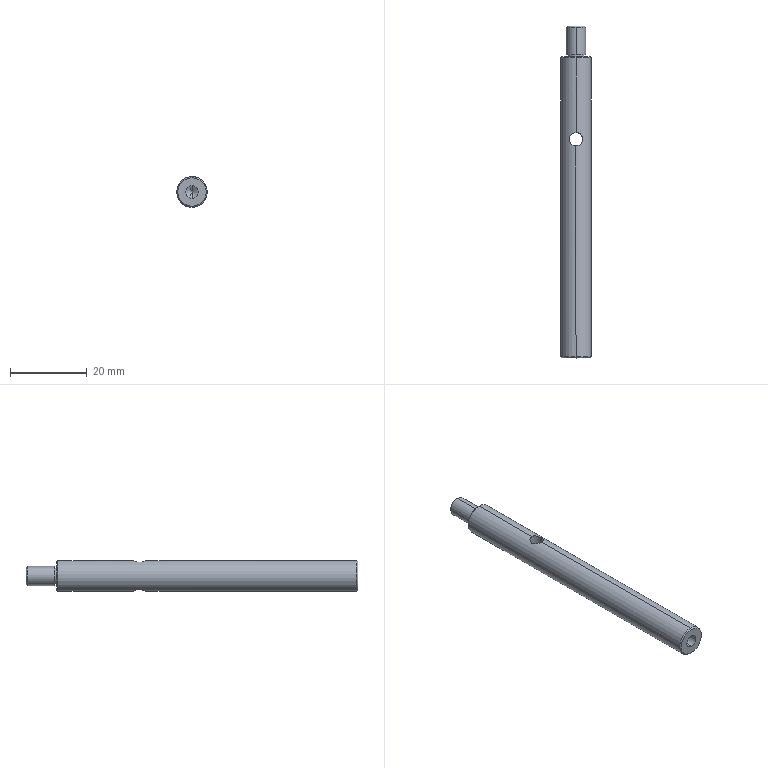Part | SolidWorks | features ICE 2, Chamfer 1, Extrusion 1, HoleWzd 1, RevCut 1 | 1 solid | 22 faces | box 8 x 86.5 x 8 mm | volume 3934 mm3 | cylinder 10 | cone 8 | plane 4 | commonest cylinder face diameters 3.3 x2 3.5 x2 4.4 x2 5 x2 8 x2
STEP:
#1=CARTESIAN_POINT('',(0.,86.2,-2.5));
#2=VERTEX_POINT('',#1);
#3=CARTESIAN_POINT('',(0.,86.2,2.5));
#4=VERTEX_POINT('',#3);
#5=CARTESIAN_POINT('',(0.,86.2,0.));
#6=DIRECTION('',(0.,-1.,0.));
#7=DIRECTION('',(0.,0.,1.));
#8=AXIS2_PLACEMENT_3D('',#5,#6,#7);
#9=CIRCLE('',#8,2.5);
#10=EDGE_CURVE('',#2,#4,#9,.T.);
#11=ORIENTED_EDGE('',*,*,#10,.T.);
#12=CARTESIAN_POINT('',(0.,79.,2.5));
#13=VERTEX_POINT('',#12);
#14=CARTESIAN_POINT('',(0.,86.5,2.5));
#15=DIRECTION('',(0.,-1.,0.));
#16=VECTOR('',#15,1000.);
#17=LINE('',#14,#16);
#18=EDGE_CURVE('',#4,#13,#17,.T.);
#19=ORIENTED_EDGE('',*,*,#18,.T.);
#20=CARTESIAN_POINT('',(0.,79.,-2.5));
#21=VERTEX_POINT('',#20);
#22=CARTESIAN_POINT('',(0.,79.,0.));
#23=DIRECTION('',(0.,-1.,0.));
#24=DIRECTION('',(0.,0.,-1.));
#25=AXIS2_PLACEMENT_3D('',#22,#23,#24);
#26=CIRCLE('',#25,2.5);
#27=EDGE_CURVE('',#21,#13,#26,.T.);
#28=ORIENTED_EDGE('',*,*,#27,.F.);
#29=CARTESIAN_POINT('',(0.,86.5,-2.5));
#30=DIRECTION('',(0.,-1.,0.));
#31=VECTOR('',#30,1000.);
#32=LINE('',#29,#31);
#33=EDGE_CURVE('',#2,#21,#32,.T.);
#34=ORIENTED_EDGE('',*,*,#33,.F.);
#35=EDGE_LOOP('',(#11,#19,#28,#34));
#36=FACE_OUTER_BOUND('',#35,.T.);
#37=CARTESIAN_POINT('',(0.,86.5,0.));
#38=DIRECTION('',(0.,-1.,0.));
#39=DIRECTION('',(0.,0.,-1.));
#40=AXIS2_PLACEMENT_3D('',#37,#38,#39);
#41=CYLINDRICAL_SURFACE('',#40,2.5);
#42=ADVANCED_FACE('',(#36),#41,.T.);
#43=CARTESIAN_POINT('',(0.,86.5,2.2));
#44=VERTEX_POINT('',#43);
#45=CARTESIAN_POINT('',(0.,86.5,-2.2));
#46=VERTEX_POINT('',#45);
#47=CARTESIAN_POINT('',(0.,86.5,0.));
#48=DIRECTION('',(0.,1.,0.));
#49=DIRECTION('',(0.,0.,1.));
#50=AXIS2_PLACEMENT_3D('',#47,#48,#49);
#51=CIRCLE('',#50,2.2);
#52=EDGE_CURVE('',#44,#46,#51,.T.);
#53=ORIENTED_EDGE('',*,*,#52,.F.);
#54=CARTESIAN_POINT('',(0.,86.5,2.2));
#55=DIRECTION('',(0.,-0.7071,0.7071));
#56=VECTOR('',#55,1000.);
#57=LINE('',#54,#56);
#58=EDGE_CURVE('',#44,#4,#57,.T.);
#59=ORIENTED_EDGE('',*,*,#58,.T.);
#60=ORIENTED_EDGE('',*,*,#10,.F.);
#61=CARTESIAN_POINT('',(0.,86.5,-2.2));
#62=DIRECTION('',(0.,-0.7071,-0.7071));
#63=VECTOR('',#62,1000.);
#64=LINE('',#61,#63);
#65=EDGE_CURVE('',#46,#2,#64,.T.);
#66=ORIENTED_EDGE('',*,*,#65,.F.);
#67=EDGE_LOOP('',(#53,#59,#60,#66));
#68=FACE_OUTER_BOUND('',#67,.T.);
#69=CARTESIAN_POINT('',(0.,86.5,0.));
#70=DIRECTION('',(0.,-1.,0.));
#71=DIRECTION('',(0.,0.,-1.));
#72=AXIS2_PLACEMENT_3D('',#69,#70,#71);
#73=CONICAL_SURFACE('',#72,2.2,0.7854);
#74=ADVANCED_FACE('',(#68),#73,.T.);
#75=CARTESIAN_POINT('',(0.,79.,-2.2));
#76=VERTEX_POINT('',#75);
#77=CARTESIAN_POINT('',(0.,79.,2.2));
#78=VERTEX_POINT('',#77);
#79=CARTESIAN_POINT('',(0.,79.,0.));
#80=DIRECTION('',(0.,-1.,0.));
#81=DIRECTION('',(0.,0.,-1.));
#82=AXIS2_PLACEMENT_3D('',#79,#80,#81);
#83=CIRCLE('',#82,2.2);
#84=EDGE_CURVE('',#76,#78,#83,.T.);
#85=ORIENTED_EDGE('',*,*,#84,.T.);
#86=CARTESIAN_POINT('',(0.,78.5,2.2));
#87=VERTEX_POINT('',#86);
#88=CARTESIAN_POINT('',(0.,0.,2.2));
#89=DIRECTION('',(0.,-1.,0.));
#90=VECTOR('',#89,1000.);
#91=LINE('',#88,#90);
#92=EDGE_CURVE('',#78,#87,#91,.T.);
#93=ORIENTED_EDGE('',*,*,#92,.T.);
#94=CARTESIAN_POINT('',(0.,78.5,-2.2));
#95=VERTEX_POINT('',#94);
#96=CARTESIAN_POINT('',(0.,78.5,0.));
#97=DIRECTION('',(0.,-1.,0.));
#98=DIRECTION('',(0.,0.,-1.));
#99=AXIS2_PLACEMENT_3D('',#96,#97,#98);
#100=CIRCLE('',#99,2.2);
#101=EDGE_CURVE('',#95,#87,#100,.T.);
#102=ORIENTED_EDGE('',*,*,#101,.F.);
#103=CARTESIAN_POINT('',(0.,0.,-2.2));
#104=DIRECTION('',(0.,-1.,0.));
#105=VECTOR('',#104,1000.);
#106=LINE('',#103,#105);
#107=EDGE_CURVE('',#76,#95,#106,.T.);
#108=ORIENTED_EDGE('',*,*,#107,.F.);
#109=EDGE_LOOP('',(#85,#93,#102,#108));
#110=FACE_OUTER_BOUND('',#109,.T.);
#111=CARTESIAN_POINT('',(0.,0.,0.));
#112=DIRECTION('',(0.,-1.,0.));
#113=DIRECTION('',(0.,0.,-1.));
#114=AXIS2_PLACEMENT_3D('',#111,#112,#113);
#115=CYLINDRICAL_SURFACE('',#114,2.2);
#116=ADVANCED_FACE('',(#110),#115,.T.);
#117=CARTESIAN_POINT('',(-1.75,57.,-3.597));
#118=VERTEX_POINT('',#117);
#119=CARTESIAN_POINT('',(0.,55.25,-4.));
#120=VERTEX_POINT('',#119);
#121=CARTESIAN_POINT('',(-1.75,57.,-3.597));
#122=CARTESIAN_POINT('',(-1.75,56.884,-3.597));
#123=CARTESIAN_POINT('',(-1.738,56.767,-3.603));
#124=CARTESIAN_POINT('',(-1.693,56.541,-3.624));
#125=CARTESIAN_POINT('',(-1.659,56.431,-3.64));
#126=CARTESIAN_POINT('',(-1.57,56.218,-3.679));
#127=CARTESIAN_POINT('',(-1.516,56.118,-3.702));
#128=CARTESIAN_POINT('',(-1.39,55.93,-3.751));
#129=CARTESIAN_POINT('',(-1.317,55.842,-3.778));
#130=CARTESIAN_POINT('',(-1.157,55.682,-3.83));
#131=CARTESIAN_POINT('',(-1.07,55.61,-3.856));
#132=CARTESIAN_POINT('',(-0.8807,55.483,-3.903));
#133=CARTESIAN_POINT('',(-0.7792,55.429,-3.925));
#134=CARTESIAN_POINT('',(-0.4639,55.297,-3.979));
#135=CARTESIAN_POINT('',(-0.2309,55.25,-4.));
#136=CARTESIAN_POINT('',(0.,55.25,-4.));
#137=B_SPLINE_CURVE_WITH_KNOTS('',3,(#121,#122,#123,#124,#125,#126,#127,#128,#129,#130,#131,#132,#133,#134,#135,#136),.UNSPECIFIED.,.F.,.F.,(4,2,2,2,2,2,2,4),(0.002772,0.003119,0.003465,0.003811,0.004157,0.004504,0.00485,0.005542),.UNSPECIFIED.);
#138=EDGE_CURVE('',#118,#120,#137,.T.);
#139=ORIENTED_EDGE('',*,*,#138,.F.);
#140=CARTESIAN_POINT('',(-1.75,57.,3.597));
#141=VERTEX_POINT('',#140);
#142=CARTESIAN_POINT('',(-1.75,57.,-5.));
#143=DIRECTION('',(0.,0.,1.));
#144=VECTOR('',#143,1000.);
#145=LINE('',#142,#144);
#146=EDGE_CURVE('',#118,#141,#145,.T.);
#147=ORIENTED_EDGE('',*,*,#146,.T.);
#148=CARTESIAN_POINT('',(0.,55.25,4.));
#149=VERTEX_POINT('',#148);
#150=CARTESIAN_POINT('',(0.,55.25,4.));
#151=CARTESIAN_POINT('',(-0.1159,55.25,4.));
#152=CARTESIAN_POINT('',(-0.2333,55.262,3.995));
#153=CARTESIAN_POINT('',(-0.4592,55.307,3.975));
#154=CARTESIAN_POINT('',(-0.5696,55.341,3.961));
#155=CARTESIAN_POINT('',(-0.7826,55.43,3.924));
#156=CARTESIAN_POINT('',(-0.8826,55.485,3.903));
#157=CARTESIAN_POINT('',(-1.071,55.611,3.855));
#158=CARTESIAN_POINT('',(-1.16,55.684,3.829));
#159=CARTESIAN_POINT('',(-1.319,55.844,3.777));
#160=CARTESIAN_POINT('',(-1.39,55.931,3.751));
#161=CARTESIAN_POINT('',(-1.517,56.12,3.702));
#162=CARTESIAN_POINT('',(-1.571,56.222,3.679));
#163=CARTESIAN_POINT('',(-1.703,56.536,3.621));
#164=CARTESIAN_POINT('',(-1.75,56.769,3.597));
#165=CARTESIAN_POINT('',(-1.75,57.,3.597));
#166=B_SPLINE_CURVE_WITH_KNOTS('',3,(#150,#151,#152,#153,#154,#155,#156,#157,#158,#159,#160,#161,#162,#163,#164,#165),.UNSPECIFIED.,.F.,.F.,(4,2,2,2,2,2,2,4),(0.002772,0.003118,0.003464,0.003811,0.004157,0.004503,0.004849,0.005542),.UNSPECIFIED.);
#167=EDGE_CURVE('',#149,#141,#166,.T.);
#168=ORIENTED_EDGE('',*,*,#167,.F.);
#169=CARTESIAN_POINT('',(1.75,57.,3.597));
#170=VERTEX_POINT('',#169);
#171=CARTESIAN_POINT('',(1.75,57.,3.597));
#172=CARTESIAN_POINT('',(1.75,56.883,3.597));
#173=CARTESIAN_POINT('',(1.738,56.768,3.603));
#174=CARTESIAN_POINT('',(1.693,56.542,3.624));
#175=CARTESIAN_POINT('',(1.659,56.43,3.64));
#176=CARTESIAN_POINT('',(1.526,56.113,3.699));
#177=CARTESIAN_POINT('',(1.397,55.922,3.752));
#178=CARTESIAN_POINT('',(1.078,55.603,3.856));
#179=CARTESIAN_POINT('',(0.885,55.473,3.907));
#180=CARTESIAN_POINT('',(0.5694,55.341,3.961));
#181=CARTESIAN_POINT('',(0.4575,55.307,3.975));
#182=CARTESIAN_POINT('',(0.2307,55.261,3.995));
#183=CARTESIAN_POINT('',(0.116,55.25,4.));
#184=CARTESIAN_POINT('',(0.,55.25,4.));
#185=B_SPLINE_CURVE_WITH_KNOTS('',3,(#171,#172,#173,#174,#175,#176,#177,#178,#179,#180,#181,#182,#183,#184),.UNSPECIFIED.,.F.,.F.,(4,2,2,2,2,2,4),(0.,0.0003465,0.000693,0.001386,0.002079,0.002425,0.002772),.UNSPECIFIED.);
#186=EDGE_CURVE('',#170,#149,#185,.T.);
#187=ORIENTED_EDGE('',*,*,#186,.F.);
#188=CARTESIAN_POINT('',(1.75,57.,-3.597));
#189=VERTEX_POINT('',#188);
#190=CARTESIAN_POINT('',(1.75,57.,-5.));
#191=DIRECTION('',(0.,0.,1.));
#192=VECTOR('',#191,1000.);
#193=LINE('',#190,#192);
#194=EDGE_CURVE('',#189,#170,#193,.T.);
#195=ORIENTED_EDGE('',*,*,#194,.F.);
#196=CARTESIAN_POINT('',(0.,55.25,-4.));
#197=CARTESIAN_POINT('',(0.1154,55.25,-4.));
#198=CARTESIAN_POINT('',(0.2327,55.262,-3.995));
#199=CARTESIAN_POINT('',(0.4595,55.307,-3.975));
#200=CARTESIAN_POINT('',(0.5691,55.341,-3.961));
#201=CARTESIAN_POINT('',(0.8874,55.474,-3.906));
#202=CARTESIAN_POINT('',(1.079,55.603,-3.856));
#203=CARTESIAN_POINT('',(1.319,55.844,-3.777));
#204=CARTESIAN_POINT('',(1.391,55.931,-3.751));
#205=CARTESIAN_POINT('',(1.516,56.119,-3.702));
#206=CARTESIAN_POINT('',(1.571,56.221,-3.679));
#207=CARTESIAN_POINT('',(1.659,56.432,-3.64));
#208=CARTESIAN_POINT('',(1.693,56.541,-3.624));
#209=CARTESIAN_POINT('',(1.738,56.767,-3.603));
#210=CARTESIAN_POINT('',(1.75,56.885,-3.597));
#211=CARTESIAN_POINT('',(1.75,57.,-3.597));
#212=B_SPLINE_CURVE_WITH_KNOTS('',3,(#196,#197,#198,#199,#200,#201,#202,#203,#204,#205,#206,#207,#208,#209,#210,#211),.UNSPECIFIED.,.F.,.F.,(4,2,2,2,2,2,2,4),(0.005542,0.005888,0.006235,0.006927,0.007273,0.007619,0.007965,0.008311),.UNSPECIFIED.);
#213=EDGE_CURVE('',#120,#189,#212,.T.);
#214=ORIENTED_EDGE('',*,*,#213,.F.);
#215=EDGE_LOOP('',(#139,#147,#168,#187,#195,#214));
#216=FACE_OUTER_BOUND('',#215,.T.);
#217=CARTESIAN_POINT('',(0.,57.,-5.));
#218=DIRECTION('',(0.,0.,1.));
#219=DIRECTION('',(1.,0.,0.));
#220=AXIS2_PLACEMENT_3D('',#217,#218,#219);
#221=CYLINDRICAL_SURFACE('',#220,1.75);
#222=ADVANCED_FACE('',(#216),#221,.F.);
#223=CARTESIAN_POINT('',(0.,10.1,1.65));
#224=VERTEX_POINT('',#223);
#225=CARTESIAN_POINT('',(0.,10.1,-1.65));
#226=VERTEX_POINT('',#225);
#227=CARTESIAN_POINT('',(0.,10.1,0.));
#228=DIRECTION('',(0.,-1.,0.));
#229=DIRECTION('',(0.,0.,-1.));
#230=AXIS2_PLACEMENT_3D('',#227,#228,#229);
#231=CIRCLE('',#230,1.65);
#232=EDGE_CURVE('',#224,#226,#231,.T.);
#233=ORIENTED_EDGE('',*,*,#232,.F.);
#234=CARTESIAN_POINT('',(0.,0.,1.65));
#235=VERTEX_POINT('',#234);
#236=CARTESIAN_POINT('',(0.,0.,1.65));
#237=DIRECTION('',(0.,-1.,0.));
#238=VECTOR('',#237,1000.);
#239=LINE('',#236,#238);
#240=EDGE_CURVE('',#224,#235,#239,.T.);
#241=ORIENTED_EDGE('',*,*,#240,.T.);
#242=CARTESIAN_POINT('',(0.,0.,-1.65));
#243=VERTEX_POINT('',#242);
#244=CARTESIAN_POINT('',(0.,0.,0.));
#245=DIRECTION('',(0.,-1.,0.));
#246=DIRECTION('',(0.,0.,-1.));
#247=AXIS2_PLACEMENT_3D('',#244,#245,#246);
#248=CIRCLE('',#247,1.65);
#249=EDGE_CURVE('',#235,#243,#248,.T.);
#250=ORIENTED_EDGE('',*,*,#249,.T.);
#251=CARTESIAN_POINT('',(0.,0.,-1.65));
#252=DIRECTION('',(0.,-1.,0.));
#253=VECTOR('',#252,1000.);
#254=LINE('',#251,#253);
#255=EDGE_CURVE('',#226,#243,#254,.T.);
#256=ORIENTED_EDGE('',*,*,#255,.F.);
#257=EDGE_LOOP('',(#233,#241,#250,#256));
#258=FACE_OUTER_BOUND('',#257,.T.);
#259=CARTESIAN_POINT('',(0.,0.,0.));
#260=DIRECTION('',(0.,-1.,0.));
#261=DIRECTION('',(0.,0.,-1.));
#262=AXIS2_PLACEMENT_3D('',#259,#260,#261);
#263=CYLINDRICAL_SURFACE('',#262,1.65);
#264=ADVANCED_FACE('',(#258),#263,.F.);
#265=CARTESIAN_POINT('',(0.,11.091,0.));
#266=VERTEX_POINT('',#265);
#267=CARTESIAN_POINT('',(0.,10.1,-1.65));
#268=DIRECTION('',(0.,-0.515,-0.8572));
#269=VECTOR('',#268,1000.);
#270=LINE('',#267,#269);
#271=EDGE_CURVE('',#266,#226,#270,.T.);
#272=ORIENTED_EDGE('',*,*,#271,.F.);
#273=CARTESIAN_POINT('',(0.,10.1,1.65));
#274=DIRECTION('',(0.,-0.515,0.8572));
#275=VECTOR('',#274,1000.);
#276=LINE('',#273,#275);
#277=EDGE_CURVE('',#266,#224,#276,.T.);
#278=ORIENTED_EDGE('',*,*,#277,.T.);
#279=ORIENTED_EDGE('',*,*,#232,.T.);
#280=EDGE_LOOP('',(#272,#278,#279));
#281=FACE_OUTER_BOUND('',#280,.T.);
#282=CARTESIAN_POINT('',(0.,10.1,0.));
#283=DIRECTION('',(0.,-1.,0.));
#284=DIRECTION('',(0.,0.,-1.));
#285=AXIS2_PLACEMENT_3D('',#282,#283,#284);
#286=CONICAL_SURFACE('',#285,1.65,1.03);
#287=ADVANCED_FACE('',(#281),#286,.F.);
#288=CARTESIAN_POINT('',(0.,78.5,3.7));
#289=VERTEX_POINT('',#288);
#290=CARTESIAN_POINT('',(0.,78.5,-3.7));
#291=VERTEX_POINT('',#290);
#292=CARTESIAN_POINT('',(0.,78.5,0.));
#293=DIRECTION('',(0.,1.,0.));
#294=DIRECTION('',(0.,0.,1.));
#295=AXIS2_PLACEMENT_3D('',#292,#293,#294);
#296=CIRCLE('',#295,3.7);
#297=EDGE_CURVE('',#289,#291,#296,.T.);
#298=ORIENTED_EDGE('',*,*,#297,.F.);
#299=CARTESIAN_POINT('',(0.,78.2,4.));
#300=VERTEX_POINT('',#299);
#301=CARTESIAN_POINT('',(0.,78.5,3.7));
#302=DIRECTION('',(0.,-0.7071,0.7071));
#303=VECTOR('',#302,1000.);
#304=LINE('',#301,#303);
#305=EDGE_CURVE('',#289,#300,#304,.T.);
#306=ORIENTED_EDGE('',*,*,#305,.T.);
#307=CARTESIAN_POINT('',(0.,78.2,-4.));
#308=VERTEX_POINT('',#307);
#309=CARTESIAN_POINT('',(0.,78.2,0.));
#310=DIRECTION('',(0.,-1.,0.));
#311=DIRECTION('',(0.,0.,1.));
#312=AXIS2_PLACEMENT_3D('',#309,#310,#311);
#313=CIRCLE('',#312,4.);
#314=EDGE_CURVE('',#308,#300,#313,.T.);
#315=ORIENTED_EDGE('',*,*,#314,.F.);
#316=CARTESIAN_POINT('',(0.,78.5,-3.7));
#317=DIRECTION('',(0.,-0.7071,-0.7071));
#318=VECTOR('',#317,1000.);
#319=LINE('',#316,#318);
#320=EDGE_CURVE('',#291,#308,#319,.T.);
#321=ORIENTED_EDGE('',*,*,#320,.F.);
#322=EDGE_LOOP('',(#298,#306,#315,#321));
#323=FACE_OUTER_BOUND('',#322,.T.);
#324=CARTESIAN_POINT('',(0.,78.5,0.));
#325=DIRECTION('',(0.,-1.,0.));
#326=DIRECTION('',(0.,0.,-1.));
#327=AXIS2_PLACEMENT_3D('',#324,#325,#326);
#328=CONICAL_SURFACE('',#327,3.7,0.7854);
#329=ADVANCED_FACE('',(#323),#328,.T.);
#330=CARTESIAN_POINT('',(0.,0.,-3.7));
#331=VERTEX_POINT('',#330);
#332=CARTESIAN_POINT('',(0.,0.,3.7));
#333=VERTEX_POINT('',#332);
#334=CARTESIAN_POINT('',(0.,0.,0.));
#335=DIRECTION('',(0.,-1.,0.));
#336=DIRECTION('',(0.,0.,1.));
#337=AXIS2_PLACEMENT_3D('',#334,#335,#336);
#338=CIRCLE('',#337,3.7);
#339=EDGE_CURVE('',#331,#333,#338,.T.);
#340=ORIENTED_EDGE('',*,*,#339,.F.);
#341=CARTESIAN_POINT('',(0.,0.3,-4.));
#342=VERTEX_POINT('',#341);
#343=CARTESIAN_POINT('',(0.,0.3,-4.));
#344=DIRECTION('',(0.,0.7071,-0.7071));
#345=VECTOR('',#344,1000.);
#346=LINE('',#343,#345);
#347=EDGE_CURVE('',#331,#342,#346,.T.);
#348=ORIENTED_EDGE('',*,*,#347,.T.);
#349=CARTESIAN_POINT('',(0.,0.3,4.));
#350=VERTEX_POINT('',#349);
#351=CARTESIAN_POINT('',(0.,0.3,0.));
#352=DIRECTION('',(0.,1.,0.));
#353=DIRECTION('',(0.,0.,1.));
#354=AXIS2_PLACEMENT_3D('',#351,#352,#353);
#355=CIRCLE('',#354,4.);
#356=EDGE_CURVE('',#350,#342,#355,.T.);
#357=ORIENTED_EDGE('',*,*,#356,.F.);
#358=CARTESIAN_POINT('',(0.,0.3,4.));
#359=DIRECTION('',(0.,0.7071,0.7071));
#360=VECTOR('',#359,1000.);
#361=LINE('',#358,#360);
#362=EDGE_CURVE('',#333,#350,#361,.T.);
#363=ORIENTED_EDGE('',*,*,#362,.F.);
#364=EDGE_LOOP('',(#340,#348,#357,#363));
#365=FACE_OUTER_BOUND('',#364,.T.);
#366=CARTESIAN_POINT('',(0.,0.3,0.));
#367=DIRECTION('',(0.,1.,0.));
#368=DIRECTION('',(0.,0.,1.));
#369=AXIS2_PLACEMENT_3D('',#366,#367,#368);
#370=CONICAL_SURFACE('',#369,4.,0.7854);
#371=ADVANCED_FACE('',(#365),#370,.T.);
#372=ORIENTED_EDGE('',*,*,#314,.T.);
#373=CARTESIAN_POINT('',(0.,58.75,4.));
#374=VERTEX_POINT('',#373);
#375=CARTESIAN_POINT('',(0.,78.5,4.));
#376=DIRECTION('',(0.,-1.,0.));
#377=VECTOR('',#376,1000.);
#378=LINE('',#375,#377);
#379=EDGE_CURVE('',#300,#374,#378,.T.);
#380=ORIENTED_EDGE('',*,*,#379,.T.);
#381=CARTESIAN_POINT('',(0.,58.75,4.));
#382=CARTESIAN_POINT('',(0.2308,58.75,4.));
#383=CARTESIAN_POINT('',(0.4636,58.703,3.979));
#384=CARTESIAN_POINT('',(0.7803,58.571,3.925));
#385=CARTESIAN_POINT('',(0.8823,58.516,3.903));
#386=CARTESIAN_POINT('',(1.071,58.389,3.855));
#387=CARTESIAN_POINT('',(1.158,58.317,3.83));
#388=CARTESIAN_POINT('',(1.399,58.076,3.751));
#389=CARTESIAN_POINT('',(1.526,57.887,3.699));
#390=CARTESIAN_POINT('',(1.659,57.568,3.64));
#391=CARTESIAN_POINT('',(1.693,57.459,3.624));
#392=CARTESIAN_POINT('',(1.738,57.234,3.603));
#393=CARTESIAN_POINT('',(1.75,57.117,3.597));
#394=CARTESIAN_POINT('',(1.75,57.,3.597));
#395=B_SPLINE_CURVE_WITH_KNOTS('',3,(#381,#382,#383,#384,#385,#386,#387,#388,#389,#390,#391,#392,#393,#394),.UNSPECIFIED.,.F.,.F.,(4,2,2,2,2,2,4),(0.008311,0.009003,0.009348,0.009694,0.01039,0.01073,0.01108),.UNSPECIFIED.);
#396=EDGE_CURVE('',#374,#170,#395,.T.);
#397=ORIENTED_EDGE('',*,*,#396,.T.);
#398=ORIENTED_EDGE('',*,*,#186,.T.);
#399=CARTESIAN_POINT('',(0.,78.5,4.));
#400=DIRECTION('',(0.,-1.,0.));
#401=VECTOR('',#400,1000.);
#402=LINE('',#399,#401);
#403=EDGE_CURVE('',#149,#350,#402,.T.);
#404=ORIENTED_EDGE('',*,*,#403,.T.);
#405=ORIENTED_EDGE('',*,*,#356,.T.);
#406=CARTESIAN_POINT('',(0.,78.5,-4.));
#407=DIRECTION('',(0.,-1.,0.));
#408=VECTOR('',#407,1000.);
#409=LINE('',#406,#408);
#410=EDGE_CURVE('',#120,#342,#409,.T.);
#411=ORIENTED_EDGE('',*,*,#410,.F.);
#412=ORIENTED_EDGE('',*,*,#213,.T.);
#413=CARTESIAN_POINT('',(0.,58.75,-4.));
#414=VERTEX_POINT('',#413);
#415=CARTESIAN_POINT('',(1.75,57.,-3.597));
#416=CARTESIAN_POINT('',(1.75,57.231,-3.597));
#417=CARTESIAN_POINT('',(1.703,57.463,-3.621));
#418=CARTESIAN_POINT('',(1.571,57.78,-3.679));
#419=CARTESIAN_POINT('',(1.516,57.881,-3.702));
#420=CARTESIAN_POINT('',(1.39,58.069,-3.751));
#421=CARTESIAN_POINT('',(1.318,58.156,-3.777));
#422=CARTESIAN_POINT('',(1.077,58.398,-3.856));
#423=CARTESIAN_POINT('',(0.8877,58.526,-3.906));
#424=CARTESIAN_POINT('',(0.5689,58.659,-3.961));
#425=CARTESIAN_POINT('',(0.4594,58.693,-3.975));
#426=CARTESIAN_POINT('',(0.2341,58.738,-3.995));
#427=CARTESIAN_POINT('',(0.1171,58.75,-4.));
#428=CARTESIAN_POINT('',(0.,58.75,-4.));
#429=B_SPLINE_CURVE_WITH_KNOTS('',3,(#415,#416,#417,#418,#419,#420,#421,#422,#423,#424,#425,#426,#427,#428),.UNSPECIFIED.,.F.,.F.,(4,2,2,2,2,2,4),(0.008311,0.009003,0.009349,0.009695,0.01039,0.01073,0.01108),.UNSPECIFIED.);
#430=EDGE_CURVE('',#189,#414,#429,.T.);
#431=ORIENTED_EDGE('',*,*,#430,.T.);
#432=CARTESIAN_POINT('',(0.,78.5,-4.));
#433=DIRECTION('',(0.,-1.,0.));
#434=VECTOR('',#433,1000.);
#435=LINE('',#432,#434);
#436=EDGE_CURVE('',#308,#414,#435,.T.);
#437=ORIENTED_EDGE('',*,*,#436,.F.);
#438=EDGE_LOOP('',(#372,#380,#397,#398,#404,#405,#411,#412,#431,#437));
#439=FACE_OUTER_BOUND('',#438,.T.);
#440=CARTESIAN_POINT('',(0.,78.5,0.));
#441=DIRECTION('',(0.,-1.,0.));
#442=DIRECTION('',(0.,0.,-1.));
#443=AXIS2_PLACEMENT_3D('',#440,#441,#442);
#444=CYLINDRICAL_SURFACE('',#443,4.);
#445=ADVANCED_FACE('',(#439),#444,.T.);
#446=CARTESIAN_POINT('',(0.,78.5,0.));
#447=DIRECTION('',(0.,1.,0.));
#448=DIRECTION('',(0.,0.,1.));
#449=AXIS2_PLACEMENT_3D('',#446,#447,#448);
#450=CIRCLE('',#449,3.7);
#451=EDGE_CURVE('',#291,#289,#450,.T.);
#452=ORIENTED_EDGE('',*,*,#451,.T.);
#453=ORIENTED_EDGE('',*,*,#297,.T.);
#454=EDGE_LOOP('',(#452,#453));
#455=FACE_OUTER_BOUND('',#454,.T.);
#456=ORIENTED_EDGE('',*,*,#101,.T.);
#457=CARTESIAN_POINT('',(0.,78.5,0.));
#458=DIRECTION('',(0.,-1.,0.));
#459=DIRECTION('',(0.,0.,-1.));
#460=AXIS2_PLACEMENT_3D('',#457,#458,#459);
#461=CIRCLE('',#460,2.2);
#462=EDGE_CURVE('',#87,#95,#461,.T.);
#463=ORIENTED_EDGE('',*,*,#462,.T.);
#464=EDGE_LOOP('',(#456,#463));
#465=FACE_BOUND('',#464,.T.);
#466=CARTESIAN_POINT('',(0.,78.5,0.));
#467=DIRECTION('',(0.,1.,0.));
#468=DIRECTION('',(0.,0.,1.));
#469=AXIS2_PLACEMENT_3D('',#466,#467,#468);
#470=PLANE('',#469);
#471=ADVANCED_FACE('',(#455,#465),#470,.T.);
#472=ORIENTED_EDGE('',*,*,#379,.F.);
#473=CARTESIAN_POINT('',(0.,78.2,0.));
#474=DIRECTION('',(0.,-1.,0.));
#475=DIRECTION('',(0.,0.,1.));
#476=AXIS2_PLACEMENT_3D('',#473,#474,#475);
#477=CIRCLE('',#476,4.);
#478=EDGE_CURVE('',#300,#308,#477,.T.);
#479=ORIENTED_EDGE('',*,*,#478,.T.);
#480=ORIENTED_EDGE('',*,*,#436,.T.);
#481=CARTESIAN_POINT('',(0.,58.75,-4.));
#482=CARTESIAN_POINT('',(-0.1173,58.75,-4.));
#483=CARTESIAN_POINT('',(-0.2323,58.738,-3.995));
#484=CARTESIAN_POINT('',(-0.4582,58.693,-3.975));
#485=CARTESIAN_POINT('',(-0.5702,58.658,-3.961));
#486=CARTESIAN_POINT('',(-0.8875,58.526,-3.906));
#487=CARTESIAN_POINT('',(-1.08,58.396,-3.855));
#488=CARTESIAN_POINT('',(-1.398,58.076,-3.751));
#489=CARTESIAN_POINT('',(-1.527,57.884,-3.698));
#490=CARTESIAN_POINT('',(-1.659,57.569,-3.64));
#491=CARTESIAN_POINT('',(-1.693,57.457,-3.624));
#492=CARTESIAN_POINT('',(-1.739,57.231,-3.602));
#493=CARTESIAN_POINT('',(-1.75,57.116,-3.597));
#494=CARTESIAN_POINT('',(-1.75,57.,-3.597));
#495=B_SPLINE_CURVE_WITH_KNOTS('',3,(#481,#482,#483,#484,#485,#486,#487,#488,#489,#490,#491,#492,#493,#494),.UNSPECIFIED.,.F.,.F.,(4,2,2,2,2,2,4),(0.,0.0003466,0.0006931,0.001386,0.002079,0.002426,0.002772),.UNSPECIFIED.);
#496=EDGE_CURVE('',#414,#118,#495,.T.);
#497=ORIENTED_EDGE('',*,*,#496,.T.);
#498=ORIENTED_EDGE('',*,*,#138,.T.);
#499=ORIENTED_EDGE('',*,*,#410,.T.);
#500=CARTESIAN_POINT('',(0.,0.3,0.));
#501=DIRECTION('',(0.,1.,0.));
#502=DIRECTION('',(0.,0.,1.));
#503=AXIS2_PLACEMENT_3D('',#500,#501,#502);
#504=CIRCLE('',#503,4.);
#505=EDGE_CURVE('',#342,#350,#504,.T.);
#506=ORIENTED_EDGE('',*,*,#505,.T.);
#507=ORIENTED_EDGE('',*,*,#403,.F.);
#508=ORIENTED_EDGE('',*,*,#167,.T.);
#509=CARTESIAN_POINT('',(-1.75,57.,3.597));
#510=CARTESIAN_POINT('',(-1.75,57.115,3.597));
#511=CARTESIAN_POINT('',(-1.738,57.233,3.603));
#512=CARTESIAN_POINT('',(-1.693,57.459,3.624));
#513=CARTESIAN_POINT('',(-1.659,57.569,3.64));
#514=CARTESIAN_POINT('',(-1.526,57.887,3.699));
#515=CARTESIAN_POINT('',(-1.397,58.078,3.752));
#516=CARTESIAN_POINT('',(-1.157,58.318,3.83));
#517=CARTESIAN_POINT('',(-1.07,58.39,3.856));
#518=CARTESIAN_POINT('',(-0.8817,58.516,3.903));
#519=CARTESIAN_POINT('',(-0.7796,58.571,3.925));
#520=CARTESIAN_POINT('',(-0.5687,58.659,3.961));
#521=CARTESIAN_POINT('',(-0.4594,58.693,3.975));
#522=CARTESIAN_POINT('',(-0.2328,58.738,3.995));
#523=CARTESIAN_POINT('',(-0.1155,58.75,4.));
#524=CARTESIAN_POINT('',(0.,58.75,4.));
#525=B_SPLINE_CURVE_WITH_KNOTS('',3,(#509,#510,#511,#512,#513,#514,#515,#516,#517,#518,#519,#520,#521,#522,#523,#524),.UNSPECIFIED.,.F.,.F.,(4,2,2,2,2,2,2,4),(0.005542,0.005888,0.006234,0.006926,0.007272,0.007618,0.007965,0.008311),.UNSPECIFIED.);
#526=EDGE_CURVE('',#141,#374,#525,.T.);
#527=ORIENTED_EDGE('',*,*,#526,.T.);
#528=EDGE_LOOP('',(#472,#479,#480,#497,#498,#499,#506,#507,#508,#527));
#529=FACE_OUTER_BOUND('',#528,.T.);
#530=CARTESIAN_POINT('',(0.,78.5,0.));
#531=DIRECTION('',(0.,-1.,0.));
#532=DIRECTION('',(0.,0.,-1.));
#533=AXIS2_PLACEMENT_3D('',#530,#531,#532);
#534=CYLINDRICAL_SURFACE('',#533,4.);
#535=ADVANCED_FACE('',(#529),#534,.T.);
#536=CARTESIAN_POINT('',(0.,0.,0.));
#537=DIRECTION('',(0.,-1.,0.));
#538=DIRECTION('',(0.,0.,-1.));
#539=AXIS2_PLACEMENT_3D('',#536,#537,#538);
#540=CIRCLE('',#539,1.65);
#541=EDGE_CURVE('',#243,#235,#540,.T.);
#542=ORIENTED_EDGE('',*,*,#541,.F.);
#543=ORIENTED_EDGE('',*,*,#249,.F.);
#544=EDGE_LOOP('',(#542,#543));
#545=FACE_BOUND('',#544,.T.);
#546=CARTESIAN_POINT('',(0.,0.,0.));
#547=DIRECTION('',(0.,-1.,0.));
#548=DIRECTION('',(0.,0.,1.));
#549=AXIS2_PLACEMENT_3D('',#546,#547,#548);
#550=CIRCLE('',#549,3.7);
#551=EDGE_CURVE('',#333,#331,#550,.T.);
#552=ORIENTED_EDGE('',*,*,#551,.T.);
#553=ORIENTED_EDGE('',*,*,#339,.T.);
#554=EDGE_LOOP('',(#552,#553));
#555=FACE_OUTER_BOUND('',#554,.T.);
#556=CARTESIAN_POINT('',(0.,0.,0.));
#557=DIRECTION('',(0.,1.,0.));
#558=DIRECTION('',(0.,0.,1.));
#559=AXIS2_PLACEMENT_3D('',#556,#557,#558);
#560=PLANE('',#559);
#561=ADVANCED_FACE('',(#545,#555),#560,.F.);
#562=ORIENTED_EDGE('',*,*,#347,.F.);
#563=ORIENTED_EDGE('',*,*,#551,.F.);
#564=ORIENTED_EDGE('',*,*,#362,.T.);
#565=ORIENTED_EDGE('',*,*,#505,.F.);
#566=EDGE_LOOP('',(#562,#563,#564,#565));
#567=FACE_OUTER_BOUND('',#566,.T.);
#568=CARTESIAN_POINT('',(0.,0.3,0.));
#569=DIRECTION('',(0.,1.,0.));
#570=DIRECTION('',(0.,0.,1.));
#571=AXIS2_PLACEMENT_3D('',#568,#569,#570);
#572=CONICAL_SURFACE('',#571,4.,0.7854);
#573=ADVANCED_FACE('',(#567),#572,.T.);
#574=ORIENTED_EDGE('',*,*,#305,.F.);
#575=ORIENTED_EDGE('',*,*,#451,.F.);
#576=ORIENTED_EDGE('',*,*,#320,.T.);
#577=ORIENTED_EDGE('',*,*,#478,.F.);
#578=EDGE_LOOP('',(#574,#575,#576,#577));
#579=FACE_OUTER_BOUND('',#578,.T.);
#580=CARTESIAN_POINT('',(0.,78.5,0.));
#581=DIRECTION('',(0.,-1.,0.));
#582=DIRECTION('',(0.,0.,-1.));
#583=AXIS2_PLACEMENT_3D('',#580,#581,#582);
#584=CONICAL_SURFACE('',#583,3.7,0.7854);
#585=ADVANCED_FACE('',(#579),#584,.T.);
#586=ORIENTED_EDGE('',*,*,#277,.F.);
#587=ORIENTED_EDGE('',*,*,#271,.T.);
#588=CARTESIAN_POINT('',(0.,10.1,0.));
#589=DIRECTION('',(0.,-1.,0.));
#590=DIRECTION('',(0.,0.,-1.));
#591=AXIS2_PLACEMENT_3D('',#588,#589,#590);
#592=CIRCLE('',#591,1.65);
#593=EDGE_CURVE('',#226,#224,#592,.T.);
#594=ORIENTED_EDGE('',*,*,#593,.T.);
#595=EDGE_LOOP('',(#586,#587,#594));
#596=FACE_OUTER_BOUND('',#595,.T.);
#597=CARTESIAN_POINT('',(0.,10.1,0.));
#598=DIRECTION('',(0.,-1.,0.));
#599=DIRECTION('',(0.,0.,-1.));
#600=AXIS2_PLACEMENT_3D('',#597,#598,#599);
#601=CONICAL_SURFACE('',#600,1.65,1.03);
#602=ADVANCED_FACE('',(#596),#601,.F.);
#603=ORIENTED_EDGE('',*,*,#240,.F.);
#604=ORIENTED_EDGE('',*,*,#593,.F.);
#605=ORIENTED_EDGE('',*,*,#255,.T.);
#606=ORIENTED_EDGE('',*,*,#541,.T.);
#607=EDGE_LOOP('',(#603,#604,#605,#606));
#608=FACE_OUTER_BOUND('',#607,.T.);
#609=CARTESIAN_POINT('',(0.,0.,0.));
#610=DIRECTION('',(0.,-1.,0.));
#611=DIRECTION('',(0.,0.,-1.));
#612=AXIS2_PLACEMENT_3D('',#609,#610,#611);
#613=CYLINDRICAL_SURFACE('',#612,1.65);
#614=ADVANCED_FACE('',(#608),#613,.F.);
#615=ORIENTED_EDGE('',*,*,#146,.F.);
#616=ORIENTED_EDGE('',*,*,#496,.F.);
#617=ORIENTED_EDGE('',*,*,#430,.F.);
#618=ORIENTED_EDGE('',*,*,#194,.T.);
#619=ORIENTED_EDGE('',*,*,#396,.F.);
#620=ORIENTED_EDGE('',*,*,#526,.F.);
#621=EDGE_LOOP('',(#615,#616,#617,#618,#619,#620));
#622=FACE_OUTER_BOUND('',#621,.T.);
#623=CARTESIAN_POINT('',(0.,57.,-5.));
#624=DIRECTION('',(0.,0.,1.));
#625=DIRECTION('',(1.,0.,0.));
#626=AXIS2_PLACEMENT_3D('',#623,#624,#625);
#627=CYLINDRICAL_SURFACE('',#626,1.75);
#628=ADVANCED_FACE('',(#622),#627,.F.);
#629=ORIENTED_EDGE('',*,*,#84,.F.);
#630=CARTESIAN_POINT('',(0.,79.,0.));
#631=DIRECTION('',(0.,-1.,0.));
#632=DIRECTION('',(0.,0.,-1.));
#633=AXIS2_PLACEMENT_3D('',#630,#631,#632);
#634=CIRCLE('',#633,2.2);
#635=EDGE_CURVE('',#78,#76,#634,.T.);
#636=ORIENTED_EDGE('',*,*,#635,.F.);
#637=EDGE_LOOP('',(#629,#636));
#638=FACE_BOUND('',#637,.T.);
#639=ORIENTED_EDGE('',*,*,#27,.T.);
#640=CARTESIAN_POINT('',(0.,79.,0.));
#641=DIRECTION('',(0.,-1.,0.));
#642=DIRECTION('',(0.,0.,-1.));
#643=AXIS2_PLACEMENT_3D('',#640,#641,#642);
#644=CIRCLE('',#643,2.5);
#645=EDGE_CURVE('',#13,#21,#644,.T.);
#646=ORIENTED_EDGE('',*,*,#645,.T.);
#647=EDGE_LOOP('',(#639,#646));
#648=FACE_OUTER_BOUND('',#647,.T.);
#649=CARTESIAN_POINT('',(2.5,79.,0.));
#650=DIRECTION('',(0.,1.,0.));
#651=DIRECTION('',(0.,0.,1.));
#652=AXIS2_PLACEMENT_3D('',#649,#650,#651);
#653=PLANE('',#652);
#654=ADVANCED_FACE('',(#638,#648),#653,.F.);
#655=ORIENTED_EDGE('',*,*,#92,.F.);
#656=ORIENTED_EDGE('',*,*,#635,.T.);
#657=ORIENTED_EDGE('',*,*,#107,.T.);
#658=ORIENTED_EDGE('',*,*,#462,.F.);
#659=EDGE_LOOP('',(#655,#656,#657,#658));
#660=FACE_OUTER_BOUND('',#659,.T.);
#661=CARTESIAN_POINT('',(0.,0.,0.));
#662=DIRECTION('',(0.,-1.,0.));
#663=DIRECTION('',(0.,0.,-1.));
#664=AXIS2_PLACEMENT_3D('',#661,#662,#663);
#665=CYLINDRICAL_SURFACE('',#664,2.2);
#666=ADVANCED_FACE('',(#660),#665,.T.);
#667=CARTESIAN_POINT('',(0.,86.5,0.));
#668=DIRECTION('',(0.,1.,0.));
#669=DIRECTION('',(0.,0.,1.));
#670=AXIS2_PLACEMENT_3D('',#667,#668,#669);
#671=CIRCLE('',#670,2.2);
#672=EDGE_CURVE('',#46,#44,#671,.T.);
#673=ORIENTED_EDGE('',*,*,#672,.T.);
#674=ORIENTED_EDGE('',*,*,#52,.T.);
#675=EDGE_LOOP('',(#673,#674));
#676=FACE_OUTER_BOUND('',#675,.T.);
#677=CARTESIAN_POINT('',(0.,86.5,0.));
#678=DIRECTION('',(0.,1.,0.));
#679=DIRECTION('',(0.,0.,1.));
#680=AXIS2_PLACEMENT_3D('',#677,#678,#679);
#681=PLANE('',#680);
#682=ADVANCED_FACE('',(#676),#681,.T.);
#683=ORIENTED_EDGE('',*,*,#58,.F.);
#684=ORIENTED_EDGE('',*,*,#672,.F.);
#685=ORIENTED_EDGE('',*,*,#65,.T.);
#686=CARTESIAN_POINT('',(0.,86.2,0.));
#687=DIRECTION('',(0.,-1.,0.));
#688=DIRECTION('',(0.,0.,1.));
#689=AXIS2_PLACEMENT_3D('',#686,#687,#688);
#690=CIRCLE('',#689,2.5);
#691=EDGE_CURVE('',#4,#2,#690,.T.);
#692=ORIENTED_EDGE('',*,*,#691,.F.);
#693=EDGE_LOOP('',(#683,#684,#685,#692));
#694=FACE_OUTER_BOUND('',#693,.T.);
#695=CARTESIAN_POINT('',(0.,86.5,0.));
#696=DIRECTION('',(0.,-1.,0.));
#697=DIRECTION('',(0.,0.,-1.));
#698=AXIS2_PLACEMENT_3D('',#695,#696,#697);
#699=CONICAL_SURFACE('',#698,2.2,0.7854);
#700=ADVANCED_FACE('',(#694),#699,.T.);
#701=ORIENTED_EDGE('',*,*,#18,.F.);
#702=ORIENTED_EDGE('',*,*,#691,.T.);
#703=ORIENTED_EDGE('',*,*,#33,.T.);
#704=ORIENTED_EDGE('',*,*,#645,.F.);
#705=EDGE_LOOP('',(#701,#702,#703,#704));
#706=FACE_OUTER_BOUND('',#705,.T.);
#707=CARTESIAN_POINT('',(0.,86.5,0.));
#708=DIRECTION('',(0.,-1.,0.));
#709=DIRECTION('',(0.,0.,-1.));
#710=AXIS2_PLACEMENT_3D('',#707,#708,#709);
#711=CYLINDRICAL_SURFACE('',#710,2.5);
#712=ADVANCED_FACE('',(#706),#711,.T.);
#713=CLOSED_SHELL('',(#42,#74,#116,#222,#264,#287,#329,#371,#445,#471,#535,#561,#573,#585,#602,#614,#628,#654,#666,#682,#700,#712));
#714=MANIFOLD_SOLID_BREP('',#713);
#715=CARTESIAN_POINT('',(0.,0.,0.));
#716=DIRECTION('',(0.,0.,1.));
#717=DIRECTION('',(1.,0.,0.));
#718=AXIS2_PLACEMENT_3D('',#715,#716,#717);
#719=(LENGTH_UNIT()NAMED_UNIT(*)SI_UNIT(.MILLI.,.METRE.));
#720=UNCERTAINTY_MEASURE_WITH_UNIT(LENGTH_MEASURE(0.00001),#719,'','');
#721=(NAMED_UNIT(*)PLANE_ANGLE_UNIT()SI_UNIT($,.RADIAN.));
#722=(NAMED_UNIT(*)SI_UNIT($,.STERADIAN.)SOLID_ANGLE_UNIT());
#723=(GEOMETRIC_REPRESENTATION_CONTEXT(3)GLOBAL_UNCERTAINTY_ASSIGNED_CONTEXT((#720))GLOBAL_UNIT_ASSIGNED_CONTEXT((#719,#721,#722))REPRESENTATION_CONTEXT('',''));
#724=ADVANCED_BREP_SHAPE_REPRESENTATION('',(#714,#718),#723);